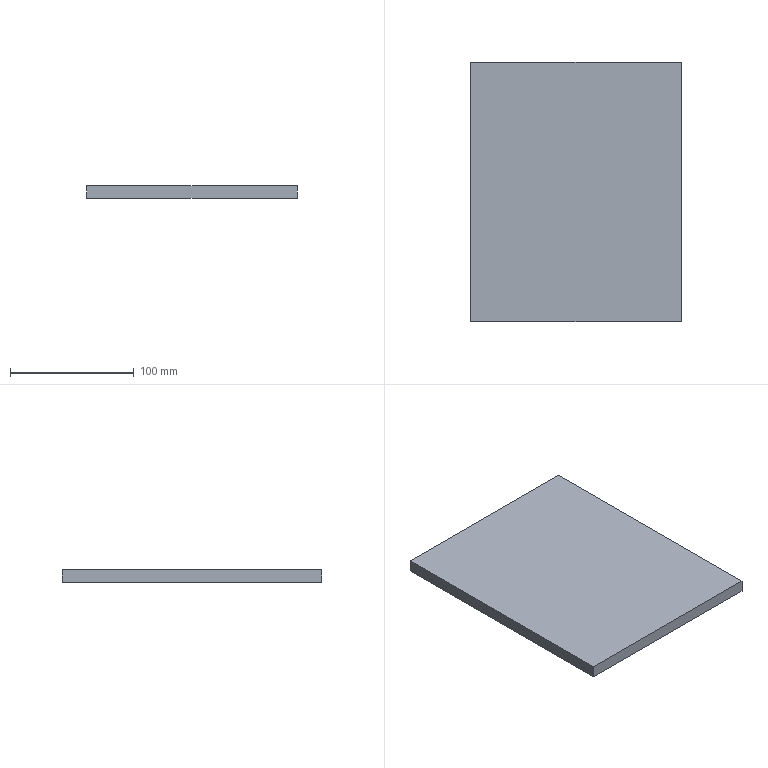Part | STEP file | 001-003-Shaft storage magazine rear plate | 1 solid | 6 faces | box 170 x 210 x 10 mm | volume 357000 mm3 | plane 6
STEP:
#1=CARTESIAN_POINT('',(0.,0.,0.));
#2=DIRECTION('',(0.,0.,1.));
#3=DIRECTION('',(1.,0.,0.));
#4=AXIS2_PLACEMENT_3D('',#1,#2,#3);
#5=CARTESIAN_POINT('',(85.,-105.,0.));
#6=VERTEX_POINT('',#5);
#7=CARTESIAN_POINT('',(85.,105.,0.));
#8=VERTEX_POINT('',#7);
#9=CARTESIAN_POINT('',(85.,-105.,0.));
#10=DIRECTION('',(0.,1.,0.));
#11=VECTOR('',#10,1.);
#12=LINE('',#9,#11);
#13=CARTESIAN_POINT('',(85.,-105.,10.));
#14=DIRECTION('',(-1.,0.,0.));
#15=DIRECTION('',(0.,0.,1.));
#16=AXIS2_PLACEMENT_3D('',#13,#14,#15);
#17=PLANE('',#16);
#18=CARTESIAN_POINT('',(-10.,0.));
#19=DIRECTION('',(0.,1.));
#20=VECTOR('',#19,1.);
#21=LINE('',#18,#20);
#22=(GEOMETRIC_REPRESENTATION_CONTEXT(2)PARAMETRIC_REPRESENTATION_CONTEXT()REPRESENTATION_CONTEXT('',''));
#23=DEFINITIONAL_REPRESENTATION('',(#21),#22);
#24=PCURVE('',#17,#23);
#25=CARTESIAN_POINT('',(0.,0.,0.));
#26=DIRECTION('',(0.,0.,-1.));
#27=DIRECTION('',(-1.,0.,0.));
#28=AXIS2_PLACEMENT_3D('',#25,#26,#27);
#29=PLANE('',#28);
#30=CARTESIAN_POINT('',(-85.,-105.));
#31=DIRECTION('',(0.,1.));
#32=VECTOR('',#31,1.);
#33=LINE('',#30,#32);
#34=(GEOMETRIC_REPRESENTATION_CONTEXT(2)PARAMETRIC_REPRESENTATION_CONTEXT()REPRESENTATION_CONTEXT('',''));
#35=DEFINITIONAL_REPRESENTATION('',(#33),#34);
#36=PCURVE('',#29,#35);
#37=SURFACE_CURVE('',#12,(#24,#36),.PCURVE_S1.);
#38=EDGE_CURVE('',#6,#8,#37,.T.);
#39=ORIENTED_EDGE('',*,*,#38,.T.);
#40=CARTESIAN_POINT('',(85.,105.,10.));
#41=VERTEX_POINT('',#40);
#42=CARTESIAN_POINT('',(85.,105.,10.));
#43=DIRECTION('',(0.,0.,-1.));
#44=VECTOR('',#43,1.);
#45=LINE('',#42,#44);
#46=CARTESIAN_POINT('',(0.,210.));
#47=DIRECTION('',(-1.,0.));
#48=VECTOR('',#47,1.);
#49=LINE('',#46,#48);
#50=(GEOMETRIC_REPRESENTATION_CONTEXT(2)PARAMETRIC_REPRESENTATION_CONTEXT()REPRESENTATION_CONTEXT('',''));
#51=DEFINITIONAL_REPRESENTATION('',(#49),#50);
#52=PCURVE('',#17,#51);
#53=CARTESIAN_POINT('',(-85.,105.,10.));
#54=DIRECTION('',(0.,-1.,0.));
#55=DIRECTION('',(0.,0.,-1.));
#56=AXIS2_PLACEMENT_3D('',#53,#54,#55);
#57=PLANE('',#56);
#58=CARTESIAN_POINT('',(0.,170.));
#59=DIRECTION('',(1.,0.));
#60=VECTOR('',#59,1.);
#61=LINE('',#58,#60);
#62=(GEOMETRIC_REPRESENTATION_CONTEXT(2)PARAMETRIC_REPRESENTATION_CONTEXT()REPRESENTATION_CONTEXT('',''));
#63=DEFINITIONAL_REPRESENTATION('',(#61),#62);
#64=PCURVE('',#57,#63);
#65=SURFACE_CURVE('',#45,(#52,#64),.PCURVE_S1.);
#66=EDGE_CURVE('',#41,#8,#65,.T.);
#67=ORIENTED_EDGE('',*,*,#66,.F.);
#68=CARTESIAN_POINT('',(85.,-105.,10.));
#69=VERTEX_POINT('',#68);
#70=CARTESIAN_POINT('',(85.,-105.,10.));
#71=DIRECTION('',(0.,1.,0.));
#72=VECTOR('',#71,1.);
#73=LINE('',#70,#72);
#74=CARTESIAN_POINT('',(0.,0.));
#75=DIRECTION('',(0.,1.));
#76=VECTOR('',#75,1.);
#77=LINE('',#74,#76);
#78=(GEOMETRIC_REPRESENTATION_CONTEXT(2)PARAMETRIC_REPRESENTATION_CONTEXT()REPRESENTATION_CONTEXT('',''));
#79=DEFINITIONAL_REPRESENTATION('',(#77),#78);
#80=PCURVE('',#17,#79);
#81=CARTESIAN_POINT('',(0.,0.,10.));
#82=DIRECTION('',(0.,0.,-1.));
#83=DIRECTION('',(-1.,0.,0.));
#84=AXIS2_PLACEMENT_3D('',#81,#82,#83);
#85=PLANE('',#84);
#86=CARTESIAN_POINT('',(-85.,-105.));
#87=DIRECTION('',(0.,1.));
#88=VECTOR('',#87,1.);
#89=LINE('',#86,#88);
#90=(GEOMETRIC_REPRESENTATION_CONTEXT(2)PARAMETRIC_REPRESENTATION_CONTEXT()REPRESENTATION_CONTEXT('',''));
#91=DEFINITIONAL_REPRESENTATION('',(#89),#90);
#92=PCURVE('',#85,#91);
#93=SURFACE_CURVE('',#73,(#80,#92),.PCURVE_S1.);
#94=EDGE_CURVE('',#69,#41,#93,.T.);
#95=ORIENTED_EDGE('',*,*,#94,.F.);
#96=CARTESIAN_POINT('',(85.,-105.,10.));
#97=DIRECTION('',(0.,0.,-1.));
#98=VECTOR('',#97,1.);
#99=LINE('',#96,#98);
#100=CARTESIAN_POINT('',(0.,0.));
#101=DIRECTION('',(-1.,0.));
#102=VECTOR('',#101,1.);
#103=LINE('',#100,#102);
#104=(GEOMETRIC_REPRESENTATION_CONTEXT(2)PARAMETRIC_REPRESENTATION_CONTEXT()REPRESENTATION_CONTEXT('',''));
#105=DEFINITIONAL_REPRESENTATION('',(#103),#104);
#106=PCURVE('',#17,#105);
#107=CARTESIAN_POINT('',(-85.,-105.,10.));
#108=DIRECTION('',(0.,1.,0.));
#109=DIRECTION('',(0.,0.,1.));
#110=AXIS2_PLACEMENT_3D('',#107,#108,#109);
#111=PLANE('',#110);
#112=CARTESIAN_POINT('',(0.,170.));
#113=DIRECTION('',(-1.,0.));
#114=VECTOR('',#113,1.);
#115=LINE('',#112,#114);
#116=(GEOMETRIC_REPRESENTATION_CONTEXT(2)PARAMETRIC_REPRESENTATION_CONTEXT()REPRESENTATION_CONTEXT('',''));
#117=DEFINITIONAL_REPRESENTATION('',(#115),#116);
#118=PCURVE('',#111,#117);
#119=SURFACE_CURVE('',#99,(#106,#118),.PCURVE_S1.);
#120=EDGE_CURVE('',#69,#6,#119,.T.);
#121=ORIENTED_EDGE('',*,*,#120,.T.);
#122=EDGE_LOOP('',(#39,#67,#95,#121));
#123=FACE_BOUND('',#122,.T.);
#124=ADVANCED_FACE('',(#123),#17,.F.);
#125=CARTESIAN_POINT('',(-85.,105.,0.));
#126=VERTEX_POINT('',#125);
#127=CARTESIAN_POINT('',(-85.,105.,0.));
#128=DIRECTION('',(-1.,0.,0.));
#129=VECTOR('',#128,1.);
#130=LINE('',#127,#129);
#131=CARTESIAN_POINT('',(10.,0.));
#132=DIRECTION('',(0.,-1.));
#133=VECTOR('',#132,1.);
#134=LINE('',#131,#133);
#135=(GEOMETRIC_REPRESENTATION_CONTEXT(2)PARAMETRIC_REPRESENTATION_CONTEXT()REPRESENTATION_CONTEXT('',''));
#136=DEFINITIONAL_REPRESENTATION('',(#134),#135);
#137=PCURVE('',#57,#136);
#138=CARTESIAN_POINT('',(85.,105.));
#139=DIRECTION('',(1.,0.));
#140=VECTOR('',#139,1.);
#141=LINE('',#138,#140);
#142=(GEOMETRIC_REPRESENTATION_CONTEXT(2)PARAMETRIC_REPRESENTATION_CONTEXT()REPRESENTATION_CONTEXT('',''));
#143=DEFINITIONAL_REPRESENTATION('',(#141),#142);
#144=PCURVE('',#29,#143);
#145=SURFACE_CURVE('',#130,(#137,#144),.PCURVE_S1.);
#146=EDGE_CURVE('',#8,#126,#145,.T.);
#147=ORIENTED_EDGE('',*,*,#146,.T.);
#148=CARTESIAN_POINT('',(-85.,105.,10.));
#149=VERTEX_POINT('',#148);
#150=CARTESIAN_POINT('',(-85.,105.,10.));
#151=DIRECTION('',(0.,0.,-1.));
#152=VECTOR('',#151,1.);
#153=LINE('',#150,#152);
#154=CARTESIAN_POINT('',(0.,0.));
#155=DIRECTION('',(1.,0.));
#156=VECTOR('',#155,1.);
#157=LINE('',#154,#156);
#158=(GEOMETRIC_REPRESENTATION_CONTEXT(2)PARAMETRIC_REPRESENTATION_CONTEXT()REPRESENTATION_CONTEXT('',''));
#159=DEFINITIONAL_REPRESENTATION('',(#157),#158);
#160=PCURVE('',#57,#159);
#161=CARTESIAN_POINT('',(-85.,-105.,10.));
#162=DIRECTION('',(1.,0.,0.));
#163=DIRECTION('',(0.,0.,-1.));
#164=AXIS2_PLACEMENT_3D('',#161,#162,#163);
#165=PLANE('',#164);
#166=CARTESIAN_POINT('',(0.,210.));
#167=DIRECTION('',(1.,0.));
#168=VECTOR('',#167,1.);
#169=LINE('',#166,#168);
#170=(GEOMETRIC_REPRESENTATION_CONTEXT(2)PARAMETRIC_REPRESENTATION_CONTEXT()REPRESENTATION_CONTEXT('',''));
#171=DEFINITIONAL_REPRESENTATION('',(#169),#170);
#172=PCURVE('',#165,#171);
#173=SURFACE_CURVE('',#153,(#160,#172),.PCURVE_S1.);
#174=EDGE_CURVE('',#149,#126,#173,.T.);
#175=ORIENTED_EDGE('',*,*,#174,.F.);
#176=CARTESIAN_POINT('',(-85.,105.,10.));
#177=DIRECTION('',(-1.,0.,0.));
#178=VECTOR('',#177,1.);
#179=LINE('',#176,#178);
#180=CARTESIAN_POINT('',(0.,0.));
#181=DIRECTION('',(0.,-1.));
#182=VECTOR('',#181,1.);
#183=LINE('',#180,#182);
#184=(GEOMETRIC_REPRESENTATION_CONTEXT(2)PARAMETRIC_REPRESENTATION_CONTEXT()REPRESENTATION_CONTEXT('',''));
#185=DEFINITIONAL_REPRESENTATION('',(#183),#184);
#186=PCURVE('',#57,#185);
#187=CARTESIAN_POINT('',(85.,105.));
#188=DIRECTION('',(1.,0.));
#189=VECTOR('',#188,1.);
#190=LINE('',#187,#189);
#191=(GEOMETRIC_REPRESENTATION_CONTEXT(2)PARAMETRIC_REPRESENTATION_CONTEXT()REPRESENTATION_CONTEXT('',''));
#192=DEFINITIONAL_REPRESENTATION('',(#190),#191);
#193=PCURVE('',#85,#192);
#194=SURFACE_CURVE('',#179,(#186,#193),.PCURVE_S1.);
#195=EDGE_CURVE('',#41,#149,#194,.T.);
#196=ORIENTED_EDGE('',*,*,#195,.F.);
#197=ORIENTED_EDGE('',*,*,#66,.T.);
#198=EDGE_LOOP('',(#147,#175,#196,#197));
#199=FACE_BOUND('',#198,.T.);
#200=ADVANCED_FACE('',(#199),#57,.F.);
#201=CARTESIAN_POINT('',(-85.,-105.,0.));
#202=VERTEX_POINT('',#201);
#203=CARTESIAN_POINT('',(-85.,-105.,0.));
#204=DIRECTION('',(0.,-1.,0.));
#205=VECTOR('',#204,1.);
#206=LINE('',#203,#205);
#207=CARTESIAN_POINT('',(10.,0.));
#208=DIRECTION('',(0.,-1.));
#209=VECTOR('',#208,1.);
#210=LINE('',#207,#209);
#211=(GEOMETRIC_REPRESENTATION_CONTEXT(2)PARAMETRIC_REPRESENTATION_CONTEXT()REPRESENTATION_CONTEXT('',''));
#212=DEFINITIONAL_REPRESENTATION('',(#210),#211);
#213=PCURVE('',#165,#212);
#214=CARTESIAN_POINT('',(85.,-105.));
#215=DIRECTION('',(0.,-1.));
#216=VECTOR('',#215,1.);
#217=LINE('',#214,#216);
#218=(GEOMETRIC_REPRESENTATION_CONTEXT(2)PARAMETRIC_REPRESENTATION_CONTEXT()REPRESENTATION_CONTEXT('',''));
#219=DEFINITIONAL_REPRESENTATION('',(#217),#218);
#220=PCURVE('',#29,#219);
#221=SURFACE_CURVE('',#206,(#213,#220),.PCURVE_S1.);
#222=EDGE_CURVE('',#126,#202,#221,.T.);
#223=ORIENTED_EDGE('',*,*,#222,.T.);
#224=CARTESIAN_POINT('',(-85.,-105.,10.));
#225=VERTEX_POINT('',#224);
#226=CARTESIAN_POINT('',(-85.,-105.,10.));
#227=DIRECTION('',(0.,0.,-1.));
#228=VECTOR('',#227,1.);
#229=LINE('',#226,#228);
#230=CARTESIAN_POINT('',(0.,0.));
#231=DIRECTION('',(1.,0.));
#232=VECTOR('',#231,1.);
#233=LINE('',#230,#232);
#234=(GEOMETRIC_REPRESENTATION_CONTEXT(2)PARAMETRIC_REPRESENTATION_CONTEXT()REPRESENTATION_CONTEXT('',''));
#235=DEFINITIONAL_REPRESENTATION('',(#233),#234);
#236=PCURVE('',#165,#235);
#237=CARTESIAN_POINT('',(0.,0.));
#238=DIRECTION('',(-1.,0.));
#239=VECTOR('',#238,1.);
#240=LINE('',#237,#239);
#241=(GEOMETRIC_REPRESENTATION_CONTEXT(2)PARAMETRIC_REPRESENTATION_CONTEXT()REPRESENTATION_CONTEXT('',''));
#242=DEFINITIONAL_REPRESENTATION('',(#240),#241);
#243=PCURVE('',#111,#242);
#244=SURFACE_CURVE('',#229,(#236,#243),.PCURVE_S1.);
#245=EDGE_CURVE('',#225,#202,#244,.T.);
#246=ORIENTED_EDGE('',*,*,#245,.F.);
#247=CARTESIAN_POINT('',(-85.,-105.,10.));
#248=DIRECTION('',(0.,-1.,0.));
#249=VECTOR('',#248,1.);
#250=LINE('',#247,#249);
#251=CARTESIAN_POINT('',(0.,0.));
#252=DIRECTION('',(0.,-1.));
#253=VECTOR('',#252,1.);
#254=LINE('',#251,#253);
#255=(GEOMETRIC_REPRESENTATION_CONTEXT(2)PARAMETRIC_REPRESENTATION_CONTEXT()REPRESENTATION_CONTEXT('',''));
#256=DEFINITIONAL_REPRESENTATION('',(#254),#255);
#257=PCURVE('',#165,#256);
#258=CARTESIAN_POINT('',(85.,-105.));
#259=DIRECTION('',(0.,-1.));
#260=VECTOR('',#259,1.);
#261=LINE('',#258,#260);
#262=(GEOMETRIC_REPRESENTATION_CONTEXT(2)PARAMETRIC_REPRESENTATION_CONTEXT()REPRESENTATION_CONTEXT('',''));
#263=DEFINITIONAL_REPRESENTATION('',(#261),#262);
#264=PCURVE('',#85,#263);
#265=SURFACE_CURVE('',#250,(#257,#264),.PCURVE_S1.);
#266=EDGE_CURVE('',#149,#225,#265,.T.);
#267=ORIENTED_EDGE('',*,*,#266,.F.);
#268=ORIENTED_EDGE('',*,*,#174,.T.);
#269=EDGE_LOOP('',(#223,#246,#267,#268));
#270=FACE_BOUND('',#269,.T.);
#271=ADVANCED_FACE('',(#270),#165,.F.);
#272=CARTESIAN_POINT('',(-85.,-105.,0.));
#273=DIRECTION('',(1.,0.,0.));
#274=VECTOR('',#273,1.);
#275=LINE('',#272,#274);
#276=CARTESIAN_POINT('',(-10.,0.));
#277=DIRECTION('',(0.,1.));
#278=VECTOR('',#277,1.);
#279=LINE('',#276,#278);
#280=(GEOMETRIC_REPRESENTATION_CONTEXT(2)PARAMETRIC_REPRESENTATION_CONTEXT()REPRESENTATION_CONTEXT('',''));
#281=DEFINITIONAL_REPRESENTATION('',(#279),#280);
#282=PCURVE('',#111,#281);
#283=CARTESIAN_POINT('',(85.,-105.));
#284=DIRECTION('',(-1.,0.));
#285=VECTOR('',#284,1.);
#286=LINE('',#283,#285);
#287=(GEOMETRIC_REPRESENTATION_CONTEXT(2)PARAMETRIC_REPRESENTATION_CONTEXT()REPRESENTATION_CONTEXT('',''));
#288=DEFINITIONAL_REPRESENTATION('',(#286),#287);
#289=PCURVE('',#29,#288);
#290=SURFACE_CURVE('',#275,(#282,#289),.PCURVE_S1.);
#291=EDGE_CURVE('',#202,#6,#290,.T.);
#292=ORIENTED_EDGE('',*,*,#291,.T.);
#293=ORIENTED_EDGE('',*,*,#120,.F.);
#294=CARTESIAN_POINT('',(-85.,-105.,10.));
#295=DIRECTION('',(1.,0.,0.));
#296=VECTOR('',#295,1.);
#297=LINE('',#294,#296);
#298=CARTESIAN_POINT('',(0.,0.));
#299=DIRECTION('',(0.,1.));
#300=VECTOR('',#299,1.);
#301=LINE('',#298,#300);
#302=(GEOMETRIC_REPRESENTATION_CONTEXT(2)PARAMETRIC_REPRESENTATION_CONTEXT()REPRESENTATION_CONTEXT('',''));
#303=DEFINITIONAL_REPRESENTATION('',(#301),#302);
#304=PCURVE('',#111,#303);
#305=CARTESIAN_POINT('',(85.,-105.));
#306=DIRECTION('',(-1.,0.));
#307=VECTOR('',#306,1.);
#308=LINE('',#305,#307);
#309=(GEOMETRIC_REPRESENTATION_CONTEXT(2)PARAMETRIC_REPRESENTATION_CONTEXT()REPRESENTATION_CONTEXT('',''));
#310=DEFINITIONAL_REPRESENTATION('',(#308),#309);
#311=PCURVE('',#85,#310);
#312=SURFACE_CURVE('',#297,(#304,#311),.PCURVE_S1.);
#313=EDGE_CURVE('',#225,#69,#312,.T.);
#314=ORIENTED_EDGE('',*,*,#313,.F.);
#315=ORIENTED_EDGE('',*,*,#245,.T.);
#316=EDGE_LOOP('',(#292,#293,#314,#315));
#317=FACE_BOUND('',#316,.T.);
#318=ADVANCED_FACE('',(#317),#111,.F.);
#319=ORIENTED_EDGE('',*,*,#94,.T.);
#320=ORIENTED_EDGE('',*,*,#195,.T.);
#321=ORIENTED_EDGE('',*,*,#266,.T.);
#322=ORIENTED_EDGE('',*,*,#313,.T.);
#323=EDGE_LOOP('',(#319,#320,#321,#322));
#324=FACE_BOUND('',#323,.T.);
#325=ADVANCED_FACE('',(#324),#85,.F.);
#326=ORIENTED_EDGE('',*,*,#38,.F.);
#327=ORIENTED_EDGE('',*,*,#291,.F.);
#328=ORIENTED_EDGE('',*,*,#222,.F.);
#329=ORIENTED_EDGE('',*,*,#146,.F.);
#330=EDGE_LOOP('',(#326,#327,#328,#329));
#331=FACE_BOUND('',#330,.T.);
#332=ADVANCED_FACE('',(#331),#29,.T.);
#333=CLOSED_SHELL('',(#124,#200,#271,#318,#325,#332));
#334=MANIFOLD_SOLID_BREP('',#333);
#335=(LENGTH_UNIT()NAMED_UNIT(*)SI_UNIT(.MILLI.,.METRE.));
#336=UNCERTAINTY_MEASURE_WITH_UNIT(LENGTH_MEASURE(0.0000001),#335,'','');
#337=(NAMED_UNIT(*)PLANE_ANGLE_UNIT()SI_UNIT($,.RADIAN.));
#338=(NAMED_UNIT(*)SI_UNIT($,.STERADIAN.)SOLID_ANGLE_UNIT());
#339=(GEOMETRIC_REPRESENTATION_CONTEXT(3)GLOBAL_UNCERTAINTY_ASSIGNED_CONTEXT((#336))GLOBAL_UNIT_ASSIGNED_CONTEXT((#335,#337,#338))REPRESENTATION_CONTEXT('',''));
#340=ADVANCED_BREP_SHAPE_REPRESENTATION('',(#4,#334),#339);